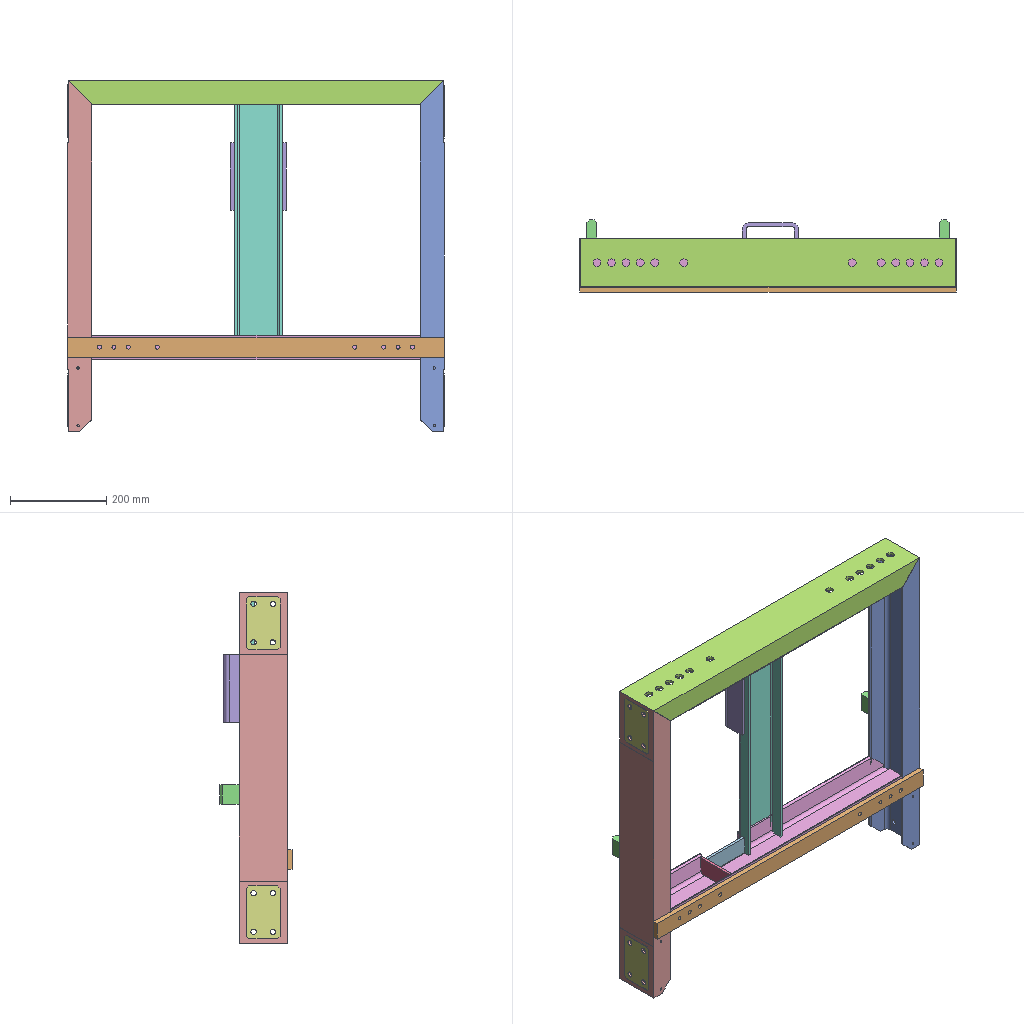Assembly | SolidWorks | 12 different items | 16 placed | box 782 x 150 x 730 mm
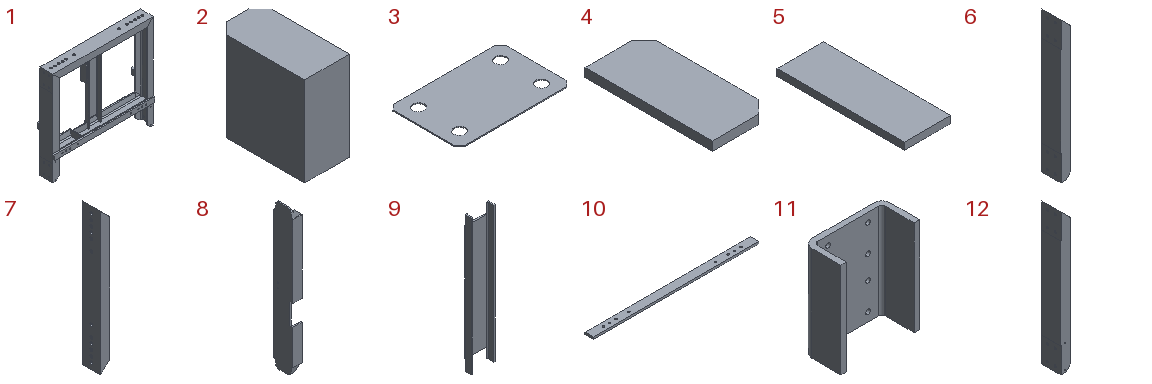Parts list (item | name | quantity | parent item | size | volume | features):
1 | (subassembly) | x1 | - | 782 x 150 x 730 mm | 4807451 mm3 | -
2 | - | x2 | in 1 | 20 x 40 x 40 mm | 31000 mm3 | features Chamfer 1, Extrusion 1
3 | - | x4 | - | 110 x 70 x 1 mm | 7270 mm3 | features Chamfer 1, Extrusion 1, ICE 1
4 | - | x1 | in 1 | 40 x 86 x 6 mm | 20206 mm3 | features Chamfer 1, Extrusion 1
5 | - | x1 | in 1 | 40 x 110 x 6 mm | 26400 mm3 | features Extrusion 1
6 | - | x1 | in 1 | 50 x 100 x 730 mm | 916470 mm3 | features ICE 3, Extrusion 1, HoleWzd 1
7 | - | x1 | in 1 | 50 x 100 x 780 mm | 980427 mm3 | features ICE 2, Extrusion 1
8 | - | x1 | in 1 | 50 x 100 x 770 mm | 903448 mm3 | features ICE 4, HoleWzd 2, Chamfer 1, Extrusion 1
9 | - | x1 | in 1 | 100 x 32 x 568 mm | 448322 mm3 | features ICE 2, Extrusion 1
10 | - | x1 | in 1 | 782 x 40 x 10 mm | 308260 mm3 | features Extrusion 1, HoleWzd 1
11 | - | x1 | in 1 | 116 x 55.5 x 140 mm | 225343 mm3 | features Extrusion 1, HoleWzd 1
12 | - | x1 | in 1 | 50 x 100 x 730 mm | 916575 mm3 | features ICE 3, HoleWzd 2, Extrusion 1
Mates (type | each side: item.copy, entity, surface, feature):
In the top assembly
Coincident | 6.1 face plane Cut-Extrude2 | 3.1 face plane Boss-Extrude1
Concentric | 6.1 edge | 3.1 edge
Coincident | 6.1 face cylinder Cut-Extrude3 | 3.1 edge
Coincident | 3.1 face plane Boss-Extrude1 | 3.2 face plane Boss-Extrude1
Concentric | 6.1 edge | 3.2 edge | 2 times
Coincident | 3.3 face plane Boss-Extrude1 | 3.4 face plane Boss-Extrude1
Coincident | 12.1 face plane Cut-Extrude2 | 3.3 face plane Boss-Extrude1
Concentric | 12.1 edge | 3.3 edge | 2 times
Concentric | 12.1 edge | 3.4 edge
Concentric | 12.1 face cylinder Cut-Extrude3 | 3.4 edge
In subassembly 1
Coincident | 12.2 face plane Cut-Extrude1 | 7.1 face plane Cut-Extrude4
Coincident | 12.2 edge | 7.1 edge
Coincident | 12.2 face plane Boss-Extrude1 | 7.1 face plane Boss-Extrude1
Coincident | 6.2 face plane Boss-Extrude1 | 7.1 face plane Boss-Extrude1
Coincident | 6.2 face plane Cut-Extrude1 | 7.1 face plane Cut-Extrude4
Coincident | 6.2 edge | 7.1 edge
Coincident | 12.2 face plane Boss-Extrude1 | 8.1 face plane Boss-Extrude1
Coincident | 7.1 face plane Boss-Extrude1 | 9.1 face plane Cut-Extrude1
Coincident | 8.1 face plane Boss-Extrude1 | 9.1 face plane Cut-Extrude2
Coincident | 8.1 face plane Boss-Extrude1 | 9.1 face plane Boss-Extrude1
Concentric | 8.1 face cylinder M10 Tapped Hole2 | 10.1 face cylinder M10 Tapped Hole3 | 2 times
Coincident | 8.1 face plane Boss-Extrude1 | 10.1 face plane Boss-Extrude1
Coincident | 9.1 face plane Boss-Extrude1 | 11.1 face plane Boss-Extrude1
DistanceDim | 11.1 face plane Boss-Extrude1 | 7.1 face plane Boss-Extrude1
DistanceDim | 11.1 face plane Boss-Extrude1 | 9.1 face plane Boss-Extrude1
Coincident | 12.2 face plane Boss-Extrude1 | 2.1 face plane Boss-Extrude1
Coincident | 6.2 face plane Boss-Extrude1 | 2.2 face plane Boss-Extrude1
Coincident | 2.2 face plane Boss-Extrude1 | 2.1 face plane Boss-Extrude1
DistanceDim | 12.2 face plane Boss-Extrude1 | 2.2 face plane Boss-Extrude1
DistanceDim | 2.1 face plane Boss-Extrude1 | 12.2 face plane Boss-Extrude1
DistanceDim | 2.2 face plane Boss-Extrude1 | 6.2 face plane Boss-Extrude1
Coincident | 8.1 face plane Boss-Extrude1 | 4.1 face plane Boss-Extrude1
Width | 12.2 face plane Boss-Extrude1 | 12.2 face plane Boss-Extrude1 | 4.1 face plane Boss-Extrude1 | 4.1 face plane Boss-Extrude1
Coincident | 8.1 face plane Cut-Extrude1 | 4.1 face plane Boss-Extrude1
Coincident | 8.1 face plane Cut-Extrude1 | 5.1 face plane Boss-Extrude1
Coincident | 4.1 face plane Boss-Extrude1 | 5.1 face plane Boss-Extrude1
Coincident | 8.1 face plane Boss-Extrude1 | 5.1 face plane Boss-Extrude1
Width | 10.1 face plane Boss-Extrude1 | 10.1 face plane Boss-Extrude1 | 6.2 face plane Boss-Extrude1 | 12.2 face plane Boss-Extrude1
Coincident | 9.1 face plane Boss-Extrude1 | 5.1 face plane Boss-Extrude1